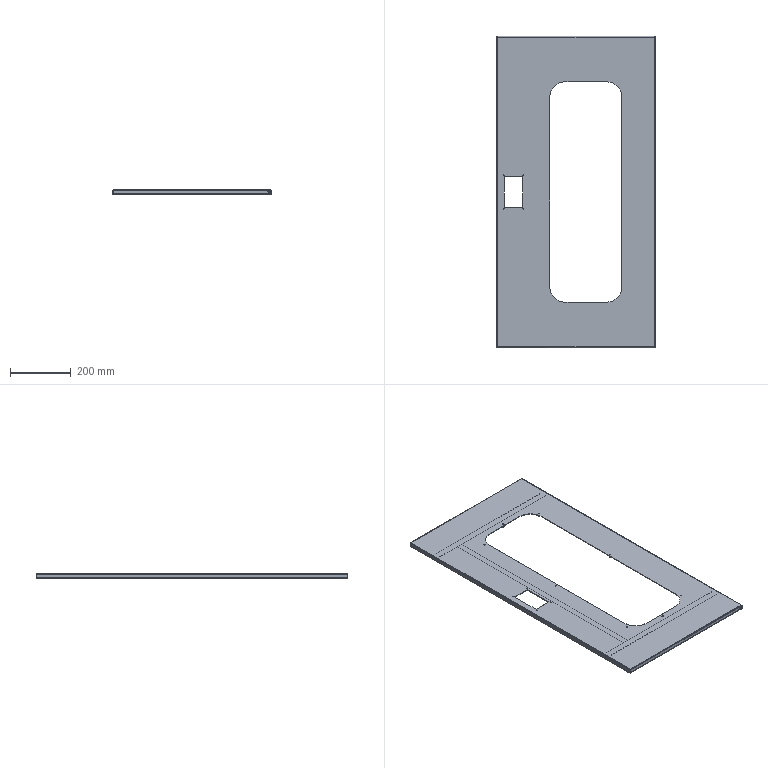Part | STEP file | 4 solids | 238 faces | box 523 x 1028 x 15 mm | volume 879625 mm3 | plane 142 | cylinder 84 | spline 12 | commonest cylinder face diameters 5 x40 1 x14 3.3 x8 4.6 x8 3.4 x6 7 x4